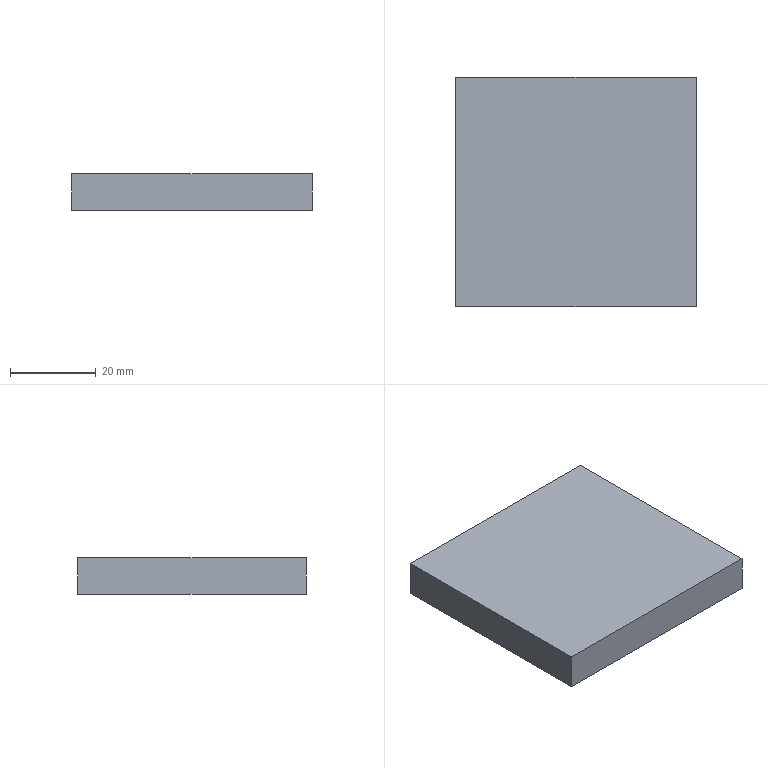NC program | NX | posted with a generic post | part box 56 x 53.3 x 8.5 mm
Lines 1400 to 2424 of 2424:
(HOLE_MILLING , TOOL : D2)
N2768 T18 M6
N2770 G54
N2772 G17 G0 G90 X-16. Y-10. S9500 M3
N2774 G43 Z30. H18
N2776 Z0.5
N2778 G94 G3 X-15.45 Y-10.55 R0.55 F1250.
N2780 X-14.9 Y-10. R0.55
N2782 X-14.9 Y-10. Z0.35 I-1.1 J0.
N2784 X-14.9 Y-10. Z0.2 I-1.1 J0.
N2786 X-14.9 Y-10. Z0.05 I-1.1 J0.
N2788 X-14.9 Y-10. Z-0.1 I-1.1 J0.
N2790 X-14.9 Y-10. Z-0.25 I-1.1 J0.
N2792 X-14.9 Y-10. Z-0.4 I-1.1 J0.
N2794 X-14.9 Y-10. Z-0.55 I-1.1 J0.
N2796 X-14.9 Y-10. Z-0.7 I-1.1 J0.
N2798 X-14.9 Y-10. Z-0.85 I-1.1 J0.
N2800 X-14.9 Y-10. Z-1. I-1.1 J0.
N2802 X-14.9 Y-10. Z-1.15 I-1.1 J0.
N2804 X-14.9 Y-10. Z-1.3 I-1.1 J0.
N2806 X-14.9 Y-10. Z-1.45 I-1.1 J0.
N2808 X-14.9 Y-10. Z-1.6 I-1.1 J0.
N2810 X-14.9 Y-10. Z-1.75 I-1.1 J0.
N2812 X-14.9 Y-10. Z-1.9 I-1.1 J0.
N2814 X-14.9 Y-10. Z-2.05 I-1.1 J0.
N2816 X-14.9 Y-10. Z-2.2 I-1.1 J0.
N2818 X-16. Y-8.9 R1.1
N2820 X-14.9 Y-10. R-1.1
N2822 X-15.45 Y-9.45 R0.55
N2824 X-16. Y-10. R0.55
N2826 G0 Z30.
N2828 X16. Y10.
N2830 Z0.5
N2832 G3 X16.55 Y9.45 R0.55
N2834 X17.1 Y10. R0.55
N2836 X17.1 Y10. Z0.35 I-1.1 J0.
N2838 X17.1 Y10. Z0.2 I-1.1 J0.
N2840 X17.1 Y10. Z0.05 I-1.1 J0.
N2842 X17.1 Y10. Z-0.1 I-1.1 J0.
N2844 X17.1 Y10. Z-0.25 I-1.1 J0.
N2846 X17.1 Y10. Z-0.4 I-1.1 J0.
N2848 X17.1 Y10. Z-0.55 I-1.1 J0.
N2850 X17.1 Y10. Z-0.7 I-1.1 J0.
N2852 X17.1 Y10. Z-0.85 I-1.1 J0.
N2854 X17.1 Y10. Z-1. I-1.1 J0.
N2856 X17.1 Y10. Z-1.15 I-1.1 J0.
N2858 X17.1 Y10. Z-1.3 I-1.1 J0.
N2860 X17.1 Y10. Z-1.45 I-1.1 J0.
N2862 X17.1 Y10. Z-1.6 I-1.1 J0.
N2864 X17.1 Y10. Z-1.75 I-1.1 J0.
N2866 X17.1 Y10. Z-1.9 I-1.1 J0.
N2868 X17.1 Y10. Z-2.05 I-1.1 J0.
N2870 X17.1 Y10. Z-2.2 I-1.1 J0.
N2872 X16. Y11.1 R1.1
N2874 X17.1 Y10. R-1.1
N2876 X16.55 Y10.55 R0.55
N2878 X16. Y10. R0.55
N2880 G0 Z30.
(ZLEVEL_PROFILE_COPY , TOOL : D2)
N2882 X-20.908 Y-9.703
N2884 Z-0.146
N2886 G1 X-20.707 Y-9.425 F1000.
N2888 G3 X-20.686 Y-9.226 R0.2
N2890 G2 X-20.995 Y-8.5 R22.65 F1200.
N2892 G1 X-21.383
N2894 G2 X-21.769 Y-8.45 R1.5
N2896 G3 X-21.962 Y-8.502 R0.2
N2898 G1 X-22.183 Y-8.724
N2900 G0 X-20.908 Y-9.703 Z-0.292
N2902 G1 X-20.707 Y-9.425 F1000.
N2904 G3 X-20.686 Y-9.226 R0.2
N2906 G2 X-20.995 Y-8.5 R22.65 F1200.
N2908 G1 X-21.383
N2910 G2 X-21.769 Y-8.45 R1.5
N2912 G3 X-21.962 Y-8.502 R0.2
N2914 G1 X-22.183 Y-8.724
N2916 G0 X-20.908 Y-9.703 Z-0.438
N2918 G1 X-20.707 Y-9.425 F1000.
N2920 G3 X-20.686 Y-9.226 R0.2
N2922 G2 X-20.995 Y-8.5 R22.65 F1200.
N2924 G1 X-21.383
N2926 G2 X-21.769 Y-8.45 R1.5
N2928 G3 X-21.962 Y-8.502 R0.2
N2930 G1 X-22.183 Y-8.724
N2932 G0 X-20.908 Y-9.703 Z-0.583
N2934 G1 X-20.707 Y-9.425 F1000.
N2936 G3 X-20.686 Y-9.226 R0.2
N2938 G2 X-20.995 Y-8.5 R22.65 F1200.
N2940 G1 X-21.383
N2942 G2 X-21.769 Y-8.45 R1.5
N2944 G3 X-21.962 Y-8.502 R0.2
N2946 G1 X-22.183 Y-8.724
N2948 G0 X-20.908 Y-9.703 Z-0.729
N2950 G1 X-20.707 Y-9.425 F1000.
N2952 G3 X-20.686 Y-9.226 R0.2
N2954 G2 X-20.995 Y-8.5 R22.65 F1200.
N2956 G1 X-21.383
N2958 G2 X-21.769 Y-8.45 R1.5
N2960 G3 X-21.962 Y-8.502 R0.2
N2962 G1 X-22.183 Y-8.724
N2964 G0 X-20.908 Y-9.703 Z-0.875
N2966 G1 X-20.707 Y-9.425 F1000.
N2968 G3 X-20.686 Y-9.226 R0.2
N2970 G2 X-20.995 Y-8.5 R22.65 F1200.
N2972 G1 X-21.383
N2974 G2 X-21.769 Y-8.45 R1.5
N2976 G3 X-21.962 Y-8.502 R0.2
N2978 G1 X-22.183 Y-8.724
N2980 G0 X-20.908 Y-9.703 Z-1.021
N2982 G1 X-20.707 Y-9.425 F1000.
N2984 G3 X-20.686 Y-9.226 R0.2
N2986 G2 X-20.995 Y-8.5 R22.65 F1200.
N2988 G1 X-21.383
N2990 G2 X-21.769 Y-8.45 R1.5
N2992 G3 X-21.962 Y-8.502 R0.2
N2994 G1 X-22.183 Y-8.724
N2996 G0 X-20.908 Y-9.703 Z-1.167
N2998 G1 X-20.707 Y-9.425 F1000.
N3000 G3 X-20.686 Y-9.226 R0.2
N3002 G2 X-20.995 Y-8.5 R22.65 F1200.
N3004 G1 X-21.383
N3006 G2 X-21.769 Y-8.45 R1.5
N3008 G3 X-21.962 Y-8.502 R0.2
N3010 G1 X-22.183 Y-8.724
N3012 G0 X-20.908 Y-9.703 Z-1.313
N3014 G1 X-20.707 Y-9.425 F1000.
N3016 G3 X-20.686 Y-9.226 R0.2
N3018 G2 X-20.995 Y-8.5 R22.65 F1200.
N3020 G1 X-21.383
N3022 G2 X-21.769 Y-8.45 R1.5
N3024 G3 X-21.962 Y-8.502 R0.2
N3026 G1 X-22.183 Y-8.724
N3028 G0 X-20.908 Y-9.703 Z-1.458
N3030 G1 X-20.707 Y-9.425 F1000.
N3032 G3 X-20.686 Y-9.226 R0.2
N3034 G2 X-20.995 Y-8.5 R22.65 F1200.
N3036 G1 X-21.383
N3038 G2 X-21.769 Y-8.45 R1.5
N3040 G3 X-21.962 Y-8.502 R0.2
N3042 G1 X-22.183 Y-8.724
N3044 G0 X-20.908 Y-9.703 Z-1.604
N3046 G1 X-20.707 Y-9.425 F1000.
N3048 G3 X-20.686 Y-9.226 R0.2
N3050 G2 X-20.995 Y-8.5 R22.65 F1200.
N3052 G1 X-21.383
N3054 G2 X-21.769 Y-8.45 R1.5
N3056 G3 X-21.962 Y-8.502 R0.2
N3058 G1 X-22.183 Y-8.724
N3060 G0 X-20.908 Y-9.703 Z-1.75
N3062 G1 X-20.707 Y-9.425 F1000.
N3064 G3 X-20.686 Y-9.226 R0.2
N3066 G2 X-20.995 Y-8.5 R22.65 F1200.
N3068 G1 X-21.383
N3070 G2 X-21.769 Y-8.45 R1.5
N3072 G3 X-21.962 Y-8.502 R0.2
N3074 G1 X-22.183 Y-8.724
N3076 G0 X-20.908 Y-9.703 Z-1.896
N3078 G1 X-20.707 Y-9.425 F1000.
N3080 G3 X-20.686 Y-9.226 R0.2
N3082 G2 X-20.995 Y-8.5 R22.65 F1200.
N3084 G1 X-21.383
N3086 G2 X-21.769 Y-8.45 R1.5
N3088 G3 X-21.962 Y-8.502 R0.2
N3090 G1 X-22.183 Y-8.724
N3092 G0 X-20.908 Y-9.703 Z-2.042
N3094 G1 X-20.707 Y-9.425 F1000.
N3096 G3 X-20.686 Y-9.226 R0.2
N3098 G2 X-20.995 Y-8.5 R22.65 F1200.
N3100 G1 X-21.383
N3102 G2 X-21.769 Y-8.45 R1.5
N3104 G3 X-21.962 Y-8.502 R0.2
N3106 G1 X-22.183 Y-8.724
N3108 G0 X-20.908 Y-9.703 Z-2.188
N3110 G1 X-20.707 Y-9.425 F1000.
N3112 G3 X-20.686 Y-9.226 R0.2
N3114 G2 X-20.995 Y-8.5 R22.65 F1200.
N3116 G1 X-21.383
N3118 G2 X-21.769 Y-8.45 R1.5
N3120 G3 X-21.962 Y-8.502 R0.2
N3122 G1 X-22.183 Y-8.724
N3124 G0 X-20.908 Y-9.703 Z-2.333
N3126 G1 X-20.707 Y-9.425 F1000.
N3128 G3 X-20.686 Y-9.226 R0.2
N3130 G2 X-20.995 Y-8.5 R22.65 F1200.
N3132 G1 X-21.383
N3134 G2 X-21.769 Y-8.45 R1.5
N3136 G3 X-21.962 Y-8.502 R0.2
N3138 G1 X-22.183 Y-8.724
N3140 G0 X-20.908 Y-9.703 Z-2.479
N3142 G1 X-20.707 Y-9.425 F1000.
N3144 G3 X-20.686 Y-9.226 R0.2
N3146 G2 X-20.995 Y-8.5 R22.65 F1200.
N3148 G1 X-21.383
N3150 G2 X-21.769 Y-8.45 R1.5
N3152 G3 X-21.962 Y-8.502 R0.2
N3154 G1 X-22.183 Y-8.724
N3156 G0 X-20.908 Y-9.703 Z-2.625
N3158 G1 X-20.707 Y-9.425 F1000.
N3160 G3 X-20.686 Y-9.226 R0.2
N3162 G2 X-20.995 Y-8.5 R22.65 F1200.
N3164 G1 X-21.383
N3166 G2 X-21.769 Y-8.45 R1.5
N3168 G3 X-21.962 Y-8.502 R0.2
N3170 G1 X-22.183 Y-8.724
N3172 G0 X-20.908 Y-9.703 Z-2.771
N3174 G1 X-20.707 Y-9.425 F1000.
N3176 G3 X-20.686 Y-9.226 R0.2
N3178 G2 X-20.995 Y-8.5 R22.65 F1200.
N3180 G1 X-21.383
N3182 G2 X-21.769 Y-8.45 R1.5
N3184 G3 X-21.962 Y-8.502 R0.2
N3186 G1 X-22.183 Y-8.724
N3188 G0 X-20.908 Y-9.703 Z-2.917
N3190 G1 X-20.707 Y-9.425 F1000.
N3192 G3 X-20.686 Y-9.226 R0.2
N3194 G2 X-20.995 Y-8.5 R22.65 F1200.
N3196 G1 X-21.383
N3198 G2 X-21.769 Y-8.45 R1.5
N3200 G3 X-21.962 Y-8.502 R0.2
N3202 G1 X-22.183 Y-8.724
N3204 G0 X-20.908 Y-9.703 Z-3.063
N3206 G1 X-20.707 Y-9.425 F1000.
N3208 G3 X-20.686 Y-9.226 R0.2
N3210 G2 X-20.995 Y-8.5 R22.65 F1200.
N3212 G1 X-21.383
N3214 G2 X-21.769 Y-8.45 R1.5
N3216 G3 X-21.962 Y-8.502 R0.2
N3218 G1 X-22.183 Y-8.724
N3220 G0 X-20.908 Y-9.703 Z-3.208
N3222 G1 X-20.707 Y-9.425 F1000.
N3224 G3 X-20.686 Y-9.226 R0.2
N3226 G2 X-20.995 Y-8.5 R22.65 F1200.
N3228 G1 X-21.383
N3230 G2 X-21.769 Y-8.45 R1.5
N3232 G3 X-21.962 Y-8.502 R0.2
N3234 G1 X-22.183 Y-8.724
N3236 G0 X-20.908 Y-9.703 Z-3.354
N3238 G1 X-20.707 Y-9.425 F1000.
N3240 G3 X-20.686 Y-9.226 R0.2
N3242 G2 X-20.995 Y-8.5 R22.65 F1200.
N3244 G1 X-21.383
N3246 G2 X-21.769 Y-8.45 R1.5
N3248 G3 X-21.962 Y-8.502 R0.2
N3250 G1 X-22.183 Y-8.724
N3252 G0 X-20.908 Y-9.703 Z-3.5
N3254 G1 X-20.707 Y-9.425 F1000.
N3256 G3 X-20.686 Y-9.226 R0.2
N3258 G2 X-20.995 Y-8.5 R22.65 F1200.
N3260 G1 X-21.383
N3262 G2 X-21.769 Y-8.45 R1.5
N3264 G3 X-21.962 Y-8.502 R0.2
N3266 G1 X-22.183 Y-8.724
N3268 G0 Z30.
N3270 Y8.724
N3272 Z-0.146
N3274 G1 X-21.962 Y8.502 F1000.
N3276 G3 X-21.769 Y8.45 R0.2
N3278 G2 X-21.383 Y8.5 R1.5 F1200.
N3280 G1 X-20.995
N3282 G2 X-20.686 Y9.226 R22.65
N3284 G3 X-20.707 Y9.425 R0.2
N3286 G1 X-20.908 Y9.703
N3288 G0 X-22.183 Y8.724 Z-0.292
N3290 G1 X-21.962 Y8.502 F1000.
N3292 G3 X-21.769 Y8.45 R0.2
N3294 G2 X-21.383 Y8.5 R1.5 F1200.
N3296 G1 X-20.995
N3298 G2 X-20.686 Y9.226 R22.65
N3300 G3 X-20.707 Y9.425 R0.2
N3302 G1 X-20.908 Y9.703
N3304 G0 X-22.183 Y8.724 Z-0.438
N3306 G1 X-21.962 Y8.502 F1000.
N3308 G3 X-21.769 Y8.45 R0.2
N3310 G2 X-21.383 Y8.5 R1.5 F1200.
N3312 G1 X-20.995
N3314 G2 X-20.686 Y9.226 R22.65
N3316 G3 X-20.707 Y9.425 R0.2
N3318 G1 X-20.908 Y9.703
N3320 G0 X-22.183 Y8.724 Z-0.583
N3322 G1 X-21.962 Y8.502 F1000.
N3324 G3 X-21.769 Y8.45 R0.2
N3326 G2 X-21.383 Y8.5 R1.5 F1200.
N3328 G1 X-20.995
N3330 G2 X-20.686 Y9.226 R22.65
N3332 G3 X-20.707 Y9.425 R0.2
N3334 G1 X-20.908 Y9.703
N3336 G0 X-22.183 Y8.724 Z-0.729
N3338 G1 X-21.962 Y8.502 F1000.
N3340 G3 X-21.769 Y8.45 R0.2
N3342 G2 X-21.383 Y8.5 R1.5 F1200.
N3344 G1 X-20.995
N3346 G2 X-20.686 Y9.226 R22.65
N3348 G3 X-20.707 Y9.425 R0.2
N3350 G1 X-20.908 Y9.703
N3352 G0 X-22.183 Y8.724 Z-0.875
N3354 G1 X-21.962 Y8.502 F1000.
N3356 G3 X-21.769 Y8.45 R0.2
N3358 G2 X-21.383 Y8.5 R1.5 F1200.
N3360 G1 X-20.995
N3362 G2 X-20.686 Y9.226 R22.65
N3364 G3 X-20.707 Y9.425 R0.2
N3366 G1 X-20.908 Y9.703
N3368 G0 X-22.183 Y8.724 Z-1.021
N3370 G1 X-21.962 Y8.502 F1000.
N3372 G3 X-21.769 Y8.45 R0.2
N3374 G2 X-21.383 Y8.5 R1.5 F1200.
N3376 G1 X-20.995
N3378 G2 X-20.686 Y9.226 R22.65
N3380 G3 X-20.707 Y9.425 R0.2
N3382 G1 X-20.908 Y9.703
N3384 G0 X-22.183 Y8.724 Z-1.167
N3386 G1 X-21.962 Y8.502 F1000.
N3388 G3 X-21.769 Y8.45 R0.2
N3390 G2 X-21.383 Y8.5 R1.5 F1200.
N3392 G1 X-20.995
N3394 G2 X-20.686 Y9.226 R22.65
N3396 G3 X-20.707 Y9.425 R0.2
N3398 G1 X-20.908 Y9.703
N3400 G0 X-22.183 Y8.724 Z-1.313
N3402 G1 X-21.962 Y8.502 F1000.
N3404 G3 X-21.769 Y8.45 R0.2
N3406 G2 X-21.383 Y8.5 R1.5 F1200.
N3408 G1 X-20.995
N3410 G2 X-20.686 Y9.226 R22.65
N3412 G3 X-20.707 Y9.425 R0.2
N3414 G1 X-20.908 Y9.703
N3416 G0 X-22.183 Y8.724 Z-1.458
N3418 G1 X-21.962 Y8.502 F1000.
N3420 G3 X-21.769 Y8.45 R0.2
N3422 G2 X-21.383 Y8.5 R1.5 F1200.
N3424 G1 X-20.995
N3426 G2 X-20.686 Y9.226 R22.65
N3428 G3 X-20.707 Y9.425 R0.2
N3430 G1 X-20.908 Y9.703
N3432 G0 X-22.183 Y8.724 Z-1.604
N3434 G1 X-21.962 Y8.502 F1000.
N3436 G3 X-21.769 Y8.45 R0.2
N3438 G2 X-21.383 Y8.5 R1.5 F1200.
N3440 G1 X-20.995
N3442 G2 X-20.686 Y9.226 R22.65
N3444 G3 X-20.707 Y9.425 R0.2
N3446 G1 X-20.908 Y9.703
N3448 G0 X-22.183 Y8.724 Z-1.75
N3450 G1 X-21.962 Y8.502 F1000.
N3452 G3 X-21.769 Y8.45 R0.2
N3454 G2 X-21.383 Y8.5 R1.5 F1200.
N3456 G1 X-20.995
N3458 G2 X-20.686 Y9.226 R22.65
N3460 G3 X-20.707 Y9.425 R0.2
N3462 G1 X-20.908 Y9.703
N3464 G0 X-22.183 Y8.724 Z-1.896
N3466 G1 X-21.962 Y8.502 F1000.
N3468 G3 X-21.769 Y8.45 R0.2
N3470 G2 X-21.383 Y8.5 R1.5 F1200.
N3472 G1 X-20.995
N3474 G2 X-20.686 Y9.226 R22.65
N3476 G3 X-20.707 Y9.425 R0.2
N3478 G1 X-20.908 Y9.703
N3480 G0 X-22.183 Y8.724 Z-2.042
N3482 G1 X-21.962 Y8.502 F1000.
N3484 G3 X-21.769 Y8.45 R0.2
N3486 G2 X-21.383 Y8.5 R1.5 F1200.
N3488 G1 X-20.995
N3490 G2 X-20.686 Y9.226 R22.65
N3492 G3 X-20.707 Y9.425 R0.2
N3494 G1 X-20.908 Y9.703
N3496 G0 X-22.183 Y8.724 Z-2.188
N3498 G1 X-21.962 Y8.502 F1000.
N3500 G3 X-21.769 Y8.45 R0.2
N3502 G2 X-21.383 Y8.5 R1.5 F1200.
N3504 G1 X-20.995
N3506 G2 X-20.686 Y9.226 R22.65
N3508 G3 X-20.707 Y9.425 R0.2
N3510 G1 X-20.908 Y9.703
N3512 G0 X-22.183 Y8.724 Z-2.333
N3514 G1 X-21.962 Y8.502 F1000.
N3516 G3 X-21.769 Y8.45 R0.2
N3518 G2 X-21.383 Y8.5 R1.5 F1200.
N3520 G1 X-20.995
N3522 G2 X-20.686 Y9.226 R22.65
N3524 G3 X-20.707 Y9.425 R0.2
N3526 G1 X-20.908 Y9.703
N3528 G0 X-22.183 Y8.724 Z-2.479
N3530 G1 X-21.962 Y8.502 F1000.
N3532 G3 X-21.769 Y8.45 R0.2
N3534 G2 X-21.383 Y8.5 R1.5 F1200.
N3536 G1 X-20.995
N3538 G2 X-20.686 Y9.226 R22.65
N3540 G3 X-20.707 Y9.425 R0.2
N3542 G1 X-20.908 Y9.703
N3544 G0 X-22.183 Y8.724 Z-2.625
N3546 G1 X-21.962 Y8.502 F1000.
N3548 G3 X-21.769 Y8.45 R0.2
N3550 G2 X-21.383 Y8.5 R1.5 F1200.
N3552 G1 X-20.995
N3554 G2 X-20.686 Y9.226 R22.65
N3556 G3 X-20.707 Y9.425 R0.2
N3558 G1 X-20.908 Y9.703
N3560 G0 X-22.183 Y8.724 Z-2.771
N3562 G1 X-21.962 Y8.502 F1000.
N3564 G3 X-21.769 Y8.45 R0.2
N3566 G2 X-21.383 Y8.5 R1.5 F1200.
N3568 G1 X-20.995
N3570 G2 X-20.686 Y9.226 R22.65
N3572 G3 X-20.707 Y9.425 R0.2
N3574 G1 X-20.908 Y9.703
N3576 G0 X-22.183 Y8.724 Z-2.917
N3578 G1 X-21.962 Y8.502 F1000.
N3580 G3 X-21.769 Y8.45 R0.2
N3582 G2 X-21.383 Y8.5 R1.5 F1200.
N3584 G1 X-20.995
N3586 G2 X-20.686 Y9.226 R22.65
N3588 G3 X-20.707 Y9.425 R0.2
N3590 G1 X-20.908 Y9.703
N3592 G0 X-22.183 Y8.724 Z-3.063
N3594 G1 X-21.962 Y8.502 F1000.
N3596 G3 X-21.769 Y8.45 R0.2
N3598 G2 X-21.383 Y8.5 R1.5 F1200.
N3600 G1 X-20.995
N3602 G2 X-20.686 Y9.226 R22.65
N3604 G3 X-20.707 Y9.425 R0.2
N3606 G1 X-20.908 Y9.703
N3608 G0 X-22.183 Y8.724 Z-3.208
N3610 G1 X-21.962 Y8.502 F1000.
N3612 G3 X-21.769 Y8.45 R0.2
N3614 G2 X-21.383 Y8.5 R1.5 F1200.
N3616 G1 X-20.995
N3618 G2 X-20.686 Y9.226 R22.65
N3620 G3 X-20.707 Y9.425 R0.2
N3622 G1 X-20.908 Y9.703
N3624 G0 X-22.183 Y8.724 Z-3.354
N3626 G1 X-21.962 Y8.502 F1000.
N3628 G3 X-21.769 Y8.45 R0.2
N3630 G2 X-21.383 Y8.5 R1.5 F1200.
N3632 G1 X-20.995
N3634 G2 X-20.686 Y9.226 R22.65
N3636 G3 X-20.707 Y9.425 R0.2
N3638 G1 X-20.908 Y9.703
N3640 G0 X-22.183 Y8.724 Z-3.5
N3642 G1 X-21.962 Y8.502 F1000.
N3644 G3 X-21.769 Y8.45 R0.2
N3646 G2 X-21.383 Y8.5 R1.5 F1200.
N3648 G1 X-20.995
N3650 G2 X-20.686 Y9.226 R22.65
N3652 G3 X-20.707 Y9.425 R0.2
N3654 G1 X-20.908 Y9.703
N3656 G0 Z30.
N3658 X20.908
N3660 Z-0.146
N3662 G1 X20.707 Y9.425 F1000.
N3664 G3 X20.686 Y9.226 R0.2
N3666 G2 X20.995 Y8.5 R22.65 F1200.
N3668 G1 X21.383
N3670 G2 X21.769 Y8.45 R1.5
N3672 G3 X21.962 Y8.502 R0.2
N3674 G1 X22.183 Y8.724
N3676 G0 X20.908 Y9.703 Z-0.292
N3678 G1 X20.707 Y9.425 F1000.
N3680 G3 X20.686 Y9.226 R0.2
N3682 G2 X20.995 Y8.5 R22.65 F1200.
N3684 G1 X21.383
N3686 G2 X21.769 Y8.45 R1.5
N3688 G3 X21.962 Y8.502 R0.2
N3690 G1 X22.183 Y8.724
N3692 G0 X20.908 Y9.703 Z-0.438
N3694 G1 X20.707 Y9.425 F1000.
N3696 G3 X20.686 Y9.226 R0.2
N3698 G2 X20.995 Y8.5 R22.65 F1200.
N3700 G1 X21.383
N3702 G2 X21.769 Y8.45 R1.5
N3704 G3 X21.962 Y8.502 R0.2
N3706 G1 X22.183 Y8.724
N3708 G0 X20.908 Y9.703 Z-0.583
N3710 G1 X20.707 Y9.425 F1000.
N3712 G3 X20.686 Y9.226 R0.2
N3714 G2 X20.995 Y8.5 R22.65 F1200.
N3716 G1 X21.383
N3718 G2 X21.769 Y8.45 R1.5
N3720 G3 X21.962 Y8.502 R0.2
N3722 G1 X22.183 Y8.724
N3724 G0 X20.908 Y9.703 Z-0.729
N3726 G1 X20.707 Y9.425 F1000.
N3728 G3 X20.686 Y9.226 R0.2
N3730 G2 X20.995 Y8.5 R22.65 F1200.
N3732 G1 X21.383
N3734 G2 X21.769 Y8.45 R1.5
N3736 G3 X21.962 Y8.502 R0.2
N3738 G1 X22.183 Y8.724
N3740 G0 X20.908 Y9.703 Z-0.875
N3742 G1 X20.707 Y9.425 F1000.
N3744 G3 X20.686 Y9.226 R0.2
N3746 G2 X20.995 Y8.5 R22.65 F1200.
N3748 G1 X21.383
N3750 G2 X21.769 Y8.45 R1.5
N3752 G3 X21.962 Y8.502 R0.2
N3754 G1 X22.183 Y8.724
N3756 G0 X20.908 Y9.703 Z-1.021
N3758 G1 X20.707 Y9.425 F1000.
N3760 G3 X20.686 Y9.226 R0.2
N3762 G2 X20.995 Y8.5 R22.65 F1200.
N3764 G1 X21.383
N3766 G2 X21.769 Y8.45 R1.5
N3768 G3 X21.962 Y8.502 R0.2
N3770 G1 X22.183 Y8.724
N3772 G0 X20.908 Y9.703 Z-1.167
N3774 G1 X20.707 Y9.425 F1000.
N3776 G3 X20.686 Y9.226 R0.2
N3778 G2 X20.995 Y8.5 R22.65 F1200.
N3780 G1 X21.383
N3782 G2 X21.769 Y8.45 R1.5
N3784 G3 X21.962 Y8.502 R0.2
N3786 G1 X22.183 Y8.724
N3788 G0 X20.908 Y9.703 Z-1.313
N3790 G1 X20.707 Y9.425 F1000.
N3792 G3 X20.686 Y9.226 R0.2
N3794 G2 X20.995 Y8.5 R22.65 F1200.
N3796 G1 X21.383
N3798 G2 X21.769 Y8.45 R1.5
N3800 G3 X21.962 Y8.502 R0.2
N3802 G1 X22.183 Y8.724
N3804 G0 X20.908 Y9.703 Z-1.458
N3806 G1 X20.707 Y9.425 F1000.
N3808 G3 X20.686 Y9.226 R0.2
N3810 G2 X20.995 Y8.5 R22.65 F1200.
N3812 G1 X21.383
N3814 G2 X21.769 Y8.45 R1.5
N3816 G3 X21.962 Y8.502 R0.2
N3818 G1 X22.183 Y8.724
N3820 G0 X20.908 Y9.703 Z-1.604
N3822 G1 X20.707 Y9.425 F1000.
N3824 G3 X20.686 Y9.226 R0.2
N3826 G2 X20.995 Y8.5 R22.65 F1200.
N3828 G1 X21.383
N3830 G2 X21.769 Y8.45 R1.5
N3832 G3 X21.962 Y8.502 R0.2
N3834 G1 X22.183 Y8.724
N3836 G0 X20.908 Y9.703 Z-1.75
N3838 G1 X20.707 Y9.425 F1000.
N3840 G3 X20.686 Y9.226 R0.2
N3842 G2 X20.995 Y8.5 R22.65 F1200.
N3844 G1 X21.383
N3846 G2 X21.769 Y8.45 R1.5
N3848 G3 X21.962 Y8.502 R0.2
N3850 G1 X22.183 Y8.724
N3852 G0 X20.908 Y9.703 Z-1.896
N3854 G1 X20.707 Y9.425 F1000.
N3856 G3 X20.686 Y9.226 R0.2
N3858 G2 X20.995 Y8.5 R22.65 F1200.
N3860 G1 X21.383
N3862 G2 X21.769 Y8.45 R1.5
N3864 G3 X21.962 Y8.502 R0.2
N3866 G1 X22.183 Y8.724
N3868 G0 X20.908 Y9.703 Z-2.042
N3870 G1 X20.707 Y9.425 F1000.
N3872 G3 X20.686 Y9.226 R0.2
N3874 G2 X20.995 Y8.5 R22.65 F1200.
N3876 G1 X21.383
N3878 G2 X21.769 Y8.45 R1.5
N3880 G3 X21.962 Y8.502 R0.2
N3882 G1 X22.183 Y8.724
N3884 G0 X20.908 Y9.703 Z-2.188
N3886 G1 X20.707 Y9.425 F1000.
N3888 G3 X20.686 Y9.226 R0.2
N3890 G2 X20.995 Y8.5 R22.65 F1200.
N3892 G1 X21.383
N3894 G2 X21.769 Y8.45 R1.5
N3896 G3 X21.962 Y8.502 R0.2
N3898 G1 X22.183 Y8.724
N3900 G0 X20.908 Y9.703 Z-2.333
N3902 G1 X20.707 Y9.425 F1000.
N3904 G3 X20.686 Y9.226 R0.2
N3906 G2 X20.995 Y8.5 R22.65 F1200.
N3908 G1 X21.383
N3910 G2 X21.769 Y8.45 R1.5
N3912 G3 X21.962 Y8.502 R0.2
N3914 G1 X22.183 Y8.724
N3916 G0 X20.908 Y9.703 Z-2.479
N3918 G1 X20.707 Y9.425 F1000.
N3920 G3 X20.686 Y9.226 R0.2
N3922 G2 X20.995 Y8.5 R22.65 F1200.
N3924 G1 X21.383
N3926 G2 X21.769 Y8.45 R1.5
N3928 G3 X21.962 Y8.502 R0.2
N3930 G1 X22.183 Y8.724
N3932 G0 X20.908 Y9.703 Z-2.625
N3934 G1 X20.707 Y9.425 F1000.
N3936 G3 X20.686 Y9.226 R0.2
N3938 G2 X20.995 Y8.5 R22.65 F1200.
N3940 G1 X21.383
N3942 G2 X21.769 Y8.45 R1.5
N3944 G3 X21.962 Y8.502 R0.2
N3946 G1 X22.183 Y8.724
N3948 G0 X20.908 Y9.703 Z-2.771
N3950 G1 X20.707 Y9.425 F1000.
N3952 G3 X20.686 Y9.226 R0.2
N3954 G2 X20.995 Y8.5 R22.65 F1200.
N3956 G1 X21.383
N3958 G2 X21.769 Y8.45 R1.5
N3960 G3 X21.962 Y8.502 R0.2
N3962 G1 X22.183 Y8.724
N3964 G0 X20.908 Y9.703 Z-2.917
N3966 G1 X20.707 Y9.425 F1000.
N3968 G3 X20.686 Y9.226 R0.2
N3970 G2 X20.995 Y8.5 R22.65 F1200.
N3972 G1 X21.383
N3974 G2 X21.769 Y8.45 R1.5
N3976 G3 X21.962 Y8.502 R0.2
N3978 G1 X22.183 Y8.724
N3980 G0 X20.908 Y9.703 Z-3.063
N3982 G1 X20.707 Y9.425 F1000.
N3984 G3 X20.686 Y9.226 R0.2
N3986 G2 X20.995 Y8.5 R22.65 F1200.
N3988 G1 X21.383
N3990 G2 X21.769 Y8.45 R1.5
N3992 G3 X21.962 Y8.502 R0.2
N3994 G1 X22.183 Y8.724
N3996 G0 X20.908 Y9.703 Z-3.208
N3998 G1 X20.707 Y9.425 F1000.
N4000 G3 X20.686 Y9.226 R0.2
N4002 G2 X20.995 Y8.5 R22.65 F1200.
N4004 G1 X21.383
N4006 G2 X21.769 Y8.45 R1.5
N4008 G3 X21.962 Y8.502 R0.2
N4010 G1 X22.183 Y8.724
N4012 G0 X20.908 Y9.703 Z-3.354
N4014 G1 X20.707 Y9.425 F1000.
N4016 G3 X20.686 Y9.226 R0.2
N4018 G2 X20.995 Y8.5 R22.65 F1200.
N4020 G1 X21.383
N4022 G2 X21.769 Y8.45 R1.5
N4024 G3 X21.962 Y8.502 R0.2
N4026 G1 X22.183 Y8.724
N4028 G0 X20.908 Y9.703 Z-3.5
N4030 G1 X20.707 Y9.425 F1000.
N4032 G3 X20.686 Y9.226 R0.2
N4034 G2 X20.995 Y8.5 R22.65 F1200.
N4036 G1 X21.383
N4038 G2 X21.769 Y8.45 R1.5
N4040 G3 X21.962 Y8.502 R0.2
N4042 G1 X22.183 Y8.724
N4044 G0 Z30.
N4046 Y-8.724
N4048 Z-0.146
N4050 G1 X21.962 Y-8.502 F1000.
N4052 G3 X21.769 Y-8.45 R0.2
N4054 G2 X21.383 Y-8.5 R1.5 F1200.
N4056 G1 X20.995
N4058 G2 X20.686 Y-9.226 R22.65
N4060 G3 X20.707 Y-9.425 R0.2
N4062 G1 X20.908 Y-9.703
N4064 G0 X22.183 Y-8.724 Z-0.292
N4066 G1 X21.962 Y-8.502 F1000.
N4068 G3 X21.769 Y-8.45 R0.2
N4070 G2 X21.383 Y-8.5 R1.5 F1200.
N4072 G1 X20.995
N4074 G2 X20.686 Y-9.226 R22.65
N4076 G3 X20.707 Y-9.425 R0.2
N4078 G1 X20.908 Y-9.703
N4080 G0 X22.183 Y-8.724 Z-0.438
N4082 G1 X21.962 Y-8.502 F1000.
N4084 G3 X21.769 Y-8.45 R0.2
N4086 G2 X21.383 Y-8.5 R1.5 F1200.
N4088 G1 X20.995
N4090 G2 X20.686 Y-9.226 R22.65
N4092 G3 X20.707 Y-9.425 R0.2
N4094 G1 X20.908 Y-9.703
N4096 G0 X22.183 Y-8.724 Z-0.583
N4098 G1 X21.962 Y-8.502 F1000.
N4100 G3 X21.769 Y-8.45 R0.2
N4102 G2 X21.383 Y-8.5 R1.5 F1200.
N4104 G1 X20.995
N4106 G2 X20.686 Y-9.226 R22.65
N4108 G3 X20.707 Y-9.425 R0.2
N4110 G1 X20.908 Y-9.703
N4112 G0 X22.183 Y-8.724 Z-0.729
N4114 G1 X21.962 Y-8.502 F1000.
N4116 G3 X21.769 Y-8.45 R0.2
N4118 G2 X21.383 Y-8.5 R1.5 F1200.
N4120 G1 X20.995
N4122 G2 X20.686 Y-9.226 R22.65
N4124 G3 X20.707 Y-9.425 R0.2
N4126 G1 X20.908 Y-9.703
N4128 G0 X22.183 Y-8.724 Z-0.875
N4130 G1 X21.962 Y-8.502 F1000.
N4132 G3 X21.769 Y-8.45 R0.2
N4134 G2 X21.383 Y-8.5 R1.5 F1200.
N4136 G1 X20.995
N4138 G2 X20.686 Y-9.226 R22.65
N4140 G3 X20.707 Y-9.425 R0.2
N4142 G1 X20.908 Y-9.703
N4144 G0 X22.183 Y-8.724 Z-1.021
N4146 G1 X21.962 Y-8.502 F1000.
N4148 G3 X21.769 Y-8.45 R0.2
N4150 G2 X21.383 Y-8.5 R1.5 F1200.
N4152 G1 X20.995
N4154 G2 X20.686 Y-9.226 R22.65
N4156 G3 X20.707 Y-9.425 R0.2
N4158 G1 X20.908 Y-9.703
N4160 G0 X22.183 Y-8.724 Z-1.167
N4162 G1 X21.962 Y-8.502 F1000.
N4164 G3 X21.769 Y-8.45 R0.2
N4166 G2 X21.383 Y-8.5 R1.5 F1200.
N4168 G1 X20.995
N4170 G2 X20.686 Y-9.226 R22.65
N4172 G3 X20.707 Y-9.425 R0.2
N4174 G1 X20.908 Y-9.703
N4176 G0 X22.183 Y-8.724 Z-1.313
N4178 G1 X21.962 Y-8.502 F1000.
N4180 G3 X21.769 Y-8.45 R0.2
N4182 G2 X21.383 Y-8.5 R1.5 F1200.
N4184 G1 X20.995
N4186 G2 X20.686 Y-9.226 R22.65
N4188 G3 X20.707 Y-9.425 R0.2
N4190 G1 X20.908 Y-9.703
N4192 G0 X22.183 Y-8.724 Z-1.458
N4194 G1 X21.962 Y-8.502 F1000.
N4196 G3 X21.769 Y-8.45 R0.2
N4198 G2 X21.383 Y-8.5 R1.5 F1200.
N4200 G1 X20.995
N4202 G2 X20.686 Y-9.226 R22.65
N4204 G3 X20.707 Y-9.425 R0.2
N4206 G1 X20.908 Y-9.703
N4208 G0 X22.183 Y-8.724 Z-1.604
N4210 G1 X21.962 Y-8.502 F1000.
N4212 G3 X21.769 Y-8.45 R0.2
N4214 G2 X21.383 Y-8.5 R1.5 F1200.
N4216 G1 X20.995
N4218 G2 X20.686 Y-9.226 R22.65
N4220 G3 X20.707 Y-9.425 R0.2
N4222 G1 X20.908 Y-9.703
N4224 G0 X22.183 Y-8.724 Z-1.75
N4226 G1 X21.962 Y-8.502 F1000.
N4228 G3 X21.769 Y-8.45 R0.2
N4230 G2 X21.383 Y-8.5 R1.5 F1200.
N4232 G1 X20.995
N4234 G2 X20.686 Y-9.226 R22.65
N4236 G3 X20.707 Y-9.425 R0.2
N4238 G1 X20.908 Y-9.703
N4240 G0 X22.183 Y-8.724 Z-1.896
N4242 G1 X21.962 Y-8.502 F1000.
N4244 G3 X21.769 Y-8.45 R0.2
N4246 G2 X21.383 Y-8.5 R1.5 F1200.
N4248 G1 X20.995
N4250 G2 X20.686 Y-9.226 R22.65
N4252 G3 X20.707 Y-9.425 R0.2
N4254 G1 X20.908 Y-9.703
N4256 G0 X22.183 Y-8.724 Z-2.042
N4258 G1 X21.962 Y-8.502 F1000.
N4260 G3 X21.769 Y-8.45 R0.2
N4262 G2 X21.383 Y-8.5 R1.5 F1200.
N4264 G1 X20.995
N4266 G2 X20.686 Y-9.226 R22.65
N4268 G3 X20.707 Y-9.425 R0.2
N4270 G1 X20.908 Y-9.703
N4272 G0 X22.183 Y-8.724 Z-2.188
N4274 G1 X21.962 Y-8.502 F1000.
N4276 G3 X21.769 Y-8.45 R0.2
N4278 G2 X21.383 Y-8.5 R1.5 F1200.
N4280 G1 X20.995
N4282 G2 X20.686 Y-9.226 R22.65
N4284 G3 X20.707 Y-9.425 R0.2
N4286 G1 X20.908 Y-9.703
N4288 G0 X22.183 Y-8.724 Z-2.333
N4290 G1 X21.962 Y-8.502 F1000.
N4292 G3 X21.769 Y-8.45 R0.2
N4294 G2 X21.383 Y-8.5 R1.5 F1200.
N4296 G1 X20.995
N4298 G2 X20.686 Y-9.226 R22.65
N4300 G3 X20.707 Y-9.425 R0.2
N4302 G1 X20.908 Y-9.703
N4304 G0 X22.183 Y-8.724 Z-2.479
N4306 G1 X21.962 Y-8.502 F1000.
N4308 G3 X21.769 Y-8.45 R0.2
N4310 G2 X21.383 Y-8.5 R1.5 F1200.
N4312 G1 X20.995
N4314 G2 X20.686 Y-9.226 R22.65
N4316 G3 X20.707 Y-9.425 R0.2
N4318 G1 X20.908 Y-9.703
N4320 G0 X22.183 Y-8.724 Z-2.625
N4322 G1 X21.962 Y-8.502 F1000.
N4324 G3 X21.769 Y-8.45 R0.2
N4326 G2 X21.383 Y-8.5 R1.5 F1200.
N4328 G1 X20.995
N4330 G2 X20.686 Y-9.226 R22.65
N4332 G3 X20.707 Y-9.425 R0.2
N4334 G1 X20.908 Y-9.703
N4336 G0 X22.183 Y-8.724 Z-2.771
N4338 G1 X21.962 Y-8.502 F1000.
N4340 G3 X21.769 Y-8.45 R0.2
N4342 G2 X21.383 Y-8.5 R1.5 F1200.
N4344 G1 X20.995
N4346 G2 X20.686 Y-9.226 R22.65
N4348 G3 X20.707 Y-9.425 R0.2
N4350 G1 X20.908 Y-9.703
N4352 G0 X22.183 Y-8.724 Z-2.917
N4354 G1 X21.962 Y-8.502 F1000.
N4356 G3 X21.769 Y-8.45 R0.2
N4358 G2 X21.383 Y-8.5 R1.5 F1200.
N4360 G1 X20.995
N4362 G2 X20.686 Y-9.226 R22.65
N4364 G3 X20.707 Y-9.425 R0.2
N4366 G1 X20.908 Y-9.703
N4368 G0 X22.183 Y-8.724 Z-3.063
N4370 G1 X21.962 Y-8.502 F1000.
N4372 G3 X21.769 Y-8.45 R0.2
N4374 G2 X21.383 Y-8.5 R1.5 F1200.
N4376 G1 X20.995
N4378 G2 X20.686 Y-9.226 R22.65
N4380 G3 X20.707 Y-9.425 R0.2
N4382 G1 X20.908 Y-9.703
N4384 G0 X22.183 Y-8.724 Z-3.208
N4386 G1 X21.962 Y-8.502 F1000.
N4388 G3 X21.769 Y-8.45 R0.2
N4390 G2 X21.383 Y-8.5 R1.5 F1200.
N4392 G1 X20.995
N4394 G2 X20.686 Y-9.226 R22.65
N4396 G3 X20.707 Y-9.425 R0.2
N4398 G1 X20.908 Y-9.703
N4400 G0 X22.183 Y-8.724 Z-3.354
N4402 G1 X21.962 Y-8.502 F1000.
N4404 G3 X21.769 Y-8.45 R0.2
N4406 G2 X21.383 Y-8.5 R1.5 F1200.
N4408 G1 X20.995
N4410 G2 X20.686 Y-9.226 R22.65
N4412 G3 X20.707 Y-9.425 R0.2
N4414 G1 X20.908 Y-9.703
N4416 G0 X22.183 Y-8.724 Z-3.5
N4418 G1 X21.962 Y-8.502 F1000.
N4420 G3 X21.769 Y-8.45 R0.2
N4422 G2 X21.383 Y-8.5 R1.5 F1200.
N4424 G1 X20.995
N4426 G2 X20.686 Y-9.226 R22.65
N4428 G3 X20.707 Y-9.425 R0.2
N4430 G1 X20.908 Y-9.703
N4432 G0 Z30.
N4434 M5
(PLANAR_MILL_COPY_COPY_COPY_COPY_COPY_COPY_1_COPY_1 , TOOL : D6A45)
N4436 T01 M6
N4438 G54
N4440 G17 G0 G90 X-16.7 Y-9.134 S9500 M3
N4442 G43 Z30. H1
N4444 Z0.5
N4446 G94 G1 Z-1. F1250.
N4448 G3 X-17.2 Y-10. R1.
N4450 X-16. Y-11.2 R1.2
N4452 X-17.2 Y-10. R-1.2
N4454 X-16.7 Y-10.866 R1.
N4456 G1 Z0.5
N4458 G0 Z30.
N4460 X-20.152 Y-11.223
N4462 Z0.5
N4464 G1 Z-1.
N4466 G3 X-20.099 Y-10.225 R1.
N4468 G2 X-20.902 Y-8.462 R22.55
N4470 G1 X-20.922 Y-8.392
N4472 X-20.995 Y-8.4
N4474 X-21.383
N4476 G2 X-22.714 Y-7.436 R1.4
N4478 X-22.714 Y7.436 R23.9
N4480 X-21.383 Y8.4 R1.4
N4482 G1 X-20.995
N4484 X-20.922 Y8.392
N4486 X-20.902 Y8.462
N4488 G2 X-19.147 Y11.911 R22.55
N4490 X-14.678 Y13.124 R3.4
N4492 G3 X-13.124 Y14.678 R1.15
N4494 G2 X-11.911 Y19.147 R3.4
N4496 X11.911 Y19.147 R22.55
N4498 X13.124 Y14.678 R3.4
N4500 G3 X14.678 Y13.124 R1.15
N4502 G2 X19.147 Y11.911 R3.4
N4504 X20.902 Y8.462 R22.55
N4506 G1 X20.922 Y8.392
N4508 X20.995 Y8.4
N4510 X21.383
N4512 G2 X22.714 Y7.436 R1.4
N4514 X22.714 Y-7.436 R23.9
N4516 X21.383 Y-8.4 R1.4
N4518 G1 X20.995
N4520 X20.922 Y-8.392
N4522 X20.902 Y-8.462
N4524 G2 X19.147 Y-11.911 R22.55
N4526 X14.678 Y-13.124 R3.4
N4528 G3 X13.124 Y-14.678 R1.15
N4530 G2 X11.911 Y-19.147 R3.4
N4532 X-11.911 Y-19.147 R22.55
N4534 X-13.124 Y-14.678 R3.4
N4536 G3 X-14.678 Y-13.124 R1.15
N4538 G2 X-19.147 Y-11.911 R3.4
N4540 X-20.099 Y-10.225 R22.55
N4542 G3 X-20.937 Y-9.679 R1.
N4544 G1 Z0.5
N4546 G0 Z30.
N4548 X16.7 Y9.134
N4550 Z0.5
N4552 G1 Z-1.
N4554 G3 X17.2 Y10. R1.
N4556 X16. Y11.2 R1.2
N4558 X17.2 Y10. R-1.2
N4560 X16.7 Y10.866 R1.
N4562 G1 Z0.5
N4564 G0 Z30.
N4566 X4.198 Y18.415
N4568 Z0.5
N4570 G1 X4.183 Y18.6 Z0.448
N4572 X4. Y18.583 Z0.397
N4574 X4.017 Y18.4 Z0.346
N4576 X4.2 Y18.417 Z0.296
N4578 X4.183 Y18.6 Z0.245
N4580 X4. Y18.583 Z0.194
N4582 X4.017 Y18.4 Z0.143
N4584 X4.2 Y18.417 Z0.092
N4586 X4.183 Y18.6 Z0.041
N4588 X4. Y18.583 Z-0.01
N4590 X4.017 Y18.4 Z-0.061
N4592 X4.2 Y18.417 Z-0.112
N4594 X4.183 Y18.6 Z-0.163
N4596 X4. Y18.583 Z-0.214
N4598 X4.017 Y18.4 Z-0.265
N4600 X4.2 Y18.417 Z-0.316
N4602 X4.183 Y18.6 Z-0.367
N4604 X4. Y18.583 Z-0.417
N4606 X4.017 Y18.4 Z-0.468
N4608 X4.2 Y18.417 Z-0.519
N4610 X4.183 Y18.6 Z-0.57
N4612 X4. Y18.583 Z-0.621
N4614 X4.017 Y18.4 Z-0.672
N4616 X4.2 Y18.417 Z-0.723
N4618 X4.183 Y18.6 Z-0.774
N4620 X4. Y18.583 Z-0.825
N4622 X4.017 Y18.4 Z-0.876
N4624 X4.2 Y18.417 Z-0.927
N4626 X4.183 Y18.6 Z-0.978
N4628 X4.1 Z-1.
N4630 G3 X4. Y18.5 R0.1
N4632 X4.1 Y18.6 R-0.1
N4634 G1 Z0.5
N4636 G0 Z30.
N4638 X-10.302 Y16.115
N4640 Z0.5
N4642 G1 X-10.317 Y16.3 Z0.448
N4644 X-10.5 Y16.283 Z0.397
N4646 X-10.483 Y16.1 Z0.346
N4648 X-10.3 Y16.117 Z0.296
N4650 X-10.317 Y16.3 Z0.245
N4652 X-10.5 Y16.283 Z0.194
N4654 X-10.483 Y16.1 Z0.143
N4656 X-10.3 Y16.117 Z0.092
N4658 X-10.317 Y16.3 Z0.041
N4660 X-10.5 Y16.283 Z-0.01
N4662 X-10.483 Y16.1 Z-0.061
N4664 X-10.3 Y16.117 Z-0.112
N4666 X-10.317 Y16.3 Z-0.163
N4668 X-10.5 Y16.283 Z-0.214
N4670 X-10.483 Y16.1 Z-0.265
N4672 X-10.3 Y16.117 Z-0.316
N4674 X-10.317 Y16.3 Z-0.367
N4676 X-10.5 Y16.283 Z-0.417
N4678 X-10.483 Y16.1 Z-0.468
N4680 X-10.3 Y16.117 Z-0.519
N4682 X-10.317 Y16.3 Z-0.57
N4684 X-10.5 Y16.283 Z-0.621
N4686 X-10.483 Y16.1 Z-0.672
N4688 X-10.3 Y16.117 Z-0.723
N4690 X-10.317 Y16.3 Z-0.774
N4692 X-10.5 Y16.283 Z-0.825
N4694 X-10.483 Y16.1 Z-0.876
N4696 X-10.3 Y16.117 Z-0.927
N4698 X-10.317 Y16.3 Z-0.978
N4700 X-10.4 Z-1.
N4702 G3 X-10.5 Y16.2 R0.1
N4704 X-10.4 Y16.3 R-0.1
N4706 G1 Z0.5
N4708 G0 Z30.
N4710 M5
(刀补11 , TOOL : D4)
N4712 T11 M6
N4714 G54
N4716 G17 G0 G90 X-20.476 Y-13.566 S9500 M3
N4718 G43 Z30. H11
N4720 Z-2.5
N4722 G94 G1 Z-3.5 F1000.
N4724 G41 X-20.414 Y-13.487 D11
N4726 X-20.111 Y-12.918
N4728 G3 X-20.124 Y-12.519 R0.4
N4730 G2 X-21.699 Y-9.53 R23.7 F1200.
N4732 X-23.807 Y-7.793 R2.55
N4734 X-23.807 Y7.793 R25.05
N4736 X-21.699 Y9.53 R2.55
N4738 X-20.124 Y12.519 R23.7
N4740 X-14.163 Y14.153 R4.55
N4742 G1 X-14.176 Y14.209
N4744 G2 X-12.519 Y20.124 R4.55
N4746 X12.519 Y20.124 R23.7
N4748 X14.176 Y14.209 R4.55
N4750 G1 X14.163 Y14.153
N4752 G2 X20.124 Y12.519 R4.55
N4754 X21.699 Y9.53 R23.7
N4756 X23.807 Y7.793 R2.55
N4758 X23.807 Y-7.793 R25.05
N4760 X21.699 Y-9.53 R2.55
N4762 X20.124 Y-12.519 R23.7
N4764 X14.163 Y-14.153 R4.55
N4766 X14.665 Y-16.266 R4.55
N4768 X12.519 Y-20.124 R4.55
N4770 X-12.519 Y-20.124 R23.7
N4772 X-14.665 Y-16.266 R4.55
N4774 X-14.163 Y-14.153 R4.564
N4776 X-20.124 Y-12.519 R4.55
N4778 G3 X-20.477 Y-12.33 R0.4
N4780 G1 X-21.158 Y-12.353
N4782 G40
N4784 X-21.256 Y-12.373
N4786 Z-2.5
N4788 G0 Z30.
N4790 M5
N4792 M2